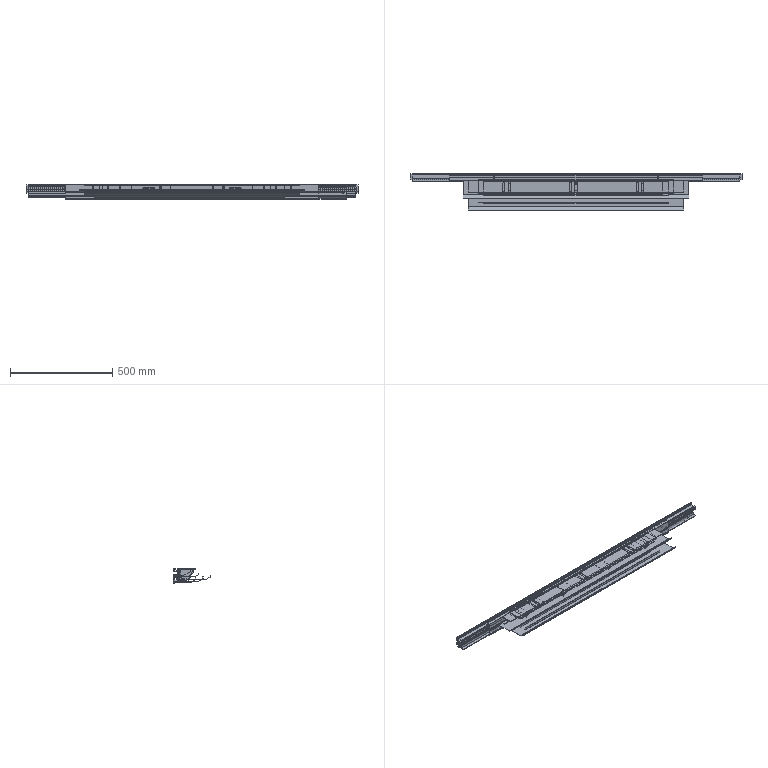Part | SolidWorks | 31 solids | 1013 faces | box 1620 x 178.321 x 70 mm | volume 5020429 mm3 | plane 675 | cylinder 338 | commonest cylinder face diameters 10 x85 9 x54 6 x48 7 x45 2 x37 3 x22